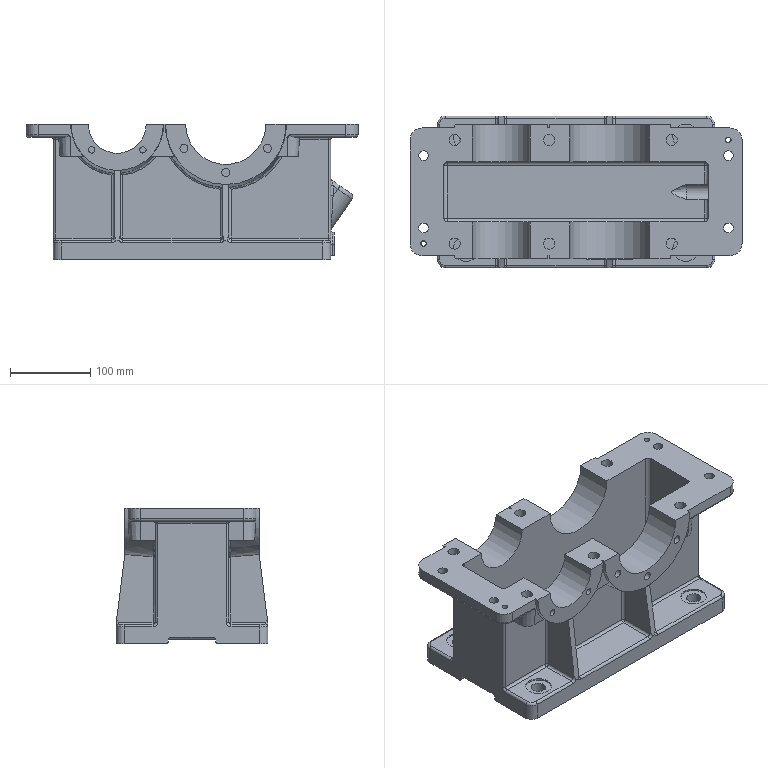Part | NX | features DATUM_CSYS 38, SKETCH 37, EXTRUDE 25, EXTRACT_FACE 22, SIMPLE HOLE 10, Instance Feature 8, HOLE PACKAGE 7, Mirror Feature 5, CBORE_HOLE 4, CPROJ 4, EXTRACT_DATUM_PLANE 4, RIB 4, BLEND 3, DATUM_PLANE 2, TAPER_HOLE 2, Pattern Feature 1, UNITE 1 | 1 solid | 286 faces | box 413 x 189 x 168.5 mm | volume 3122750 mm3 | cylinder 121 | plane 96 | torus 34 | cone 15 | sphere 12 | spline 8 | commonest cylinder face diameters 6 x59 10 x20 14 x6 20 x6 12 x5 30 x5